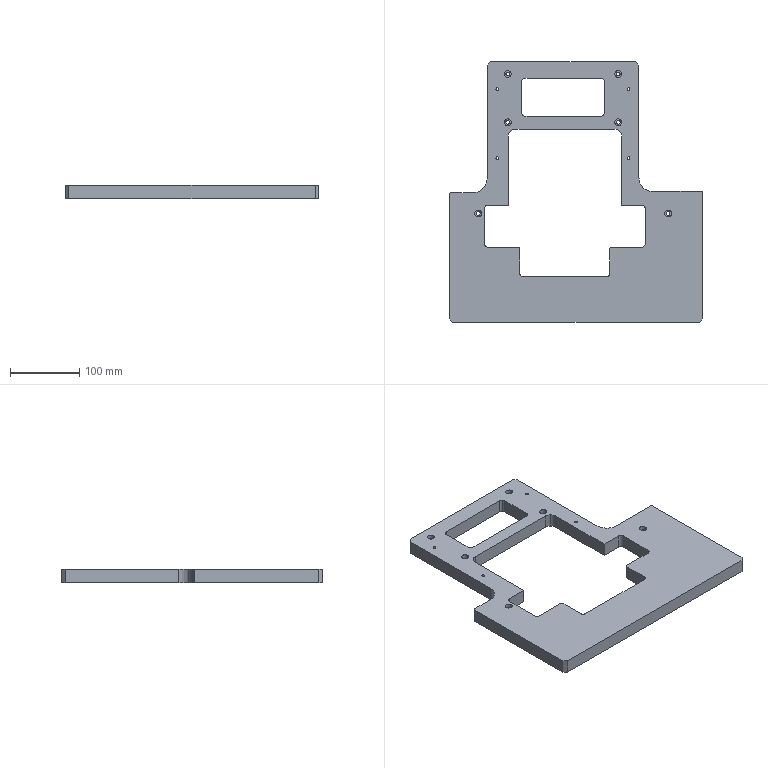Part | STEP file | ASND-0110-TCTF01-24 | 1 solid | 100 faces | box 366.812 x 377.833 x 20 mm | volume 1326662 mm3 | cylinder 64 | plane 36 | commonest cylinder face diameters 10 x28 4 x16 5.5 x12 20 x4 40 x4